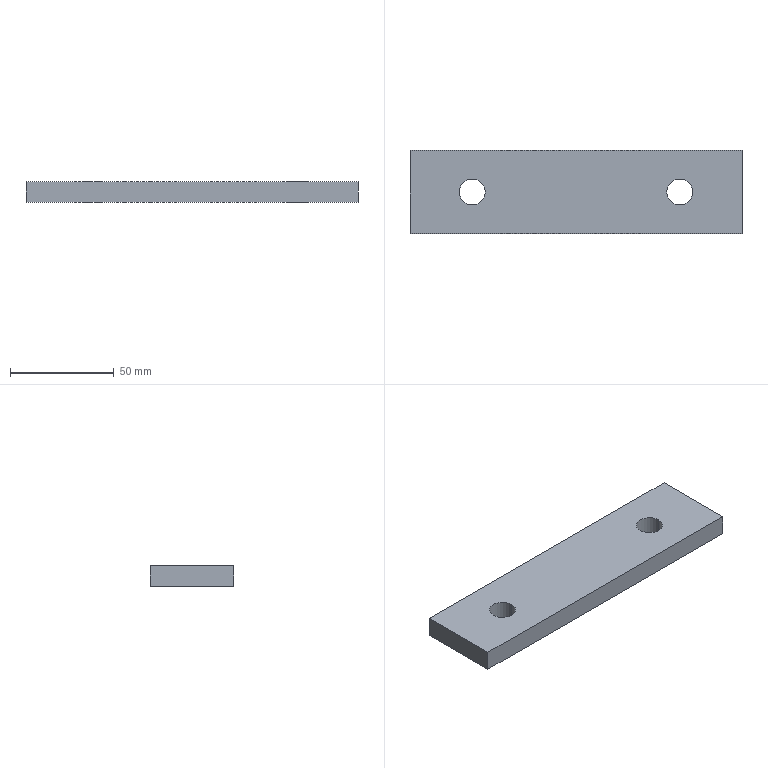Part | SolidWorks | features HoleWzd 2, Extrusion 1 | 1 solid | 10 faces | box 160 x 40 x 10 mm | volume 61546 mm3 | plane 6 | cylinder 4 | commonest cylinder face diameters 12.5 x4
STEP:
#1=CARTESIAN_POINT('',(-56.25,0.,-5.));
#2=VERTEX_POINT('',#1);
#3=CARTESIAN_POINT('',(-43.75,0.,-5.));
#4=VERTEX_POINT('',#3);
#5=CARTESIAN_POINT('',(-50.,0.,-5.));
#6=DIRECTION('',(0.,0.,1.));
#7=DIRECTION('',(1.,0.,0.));
#8=AXIS2_PLACEMENT_3D('',#5,#6,#7);
#9=CIRCLE('',#8,6.25);
#10=EDGE_CURVE('',#2,#4,#9,.T.);
#11=ORIENTED_EDGE('',*,*,#10,.F.);
#12=CARTESIAN_POINT('',(-56.25,0.,5.));
#13=VERTEX_POINT('',#12);
#14=CARTESIAN_POINT('',(-56.25,0.,5.));
#15=DIRECTION('',(0.,0.,1.));
#16=VECTOR('',#15,1000.);
#17=LINE('',#14,#16);
#18=EDGE_CURVE('',#2,#13,#17,.T.);
#19=ORIENTED_EDGE('',*,*,#18,.T.);
#20=CARTESIAN_POINT('',(-43.75,0.,5.));
#21=VERTEX_POINT('',#20);
#22=CARTESIAN_POINT('',(-50.,0.,5.));
#23=DIRECTION('',(0.,0.,1.));
#24=DIRECTION('',(1.,0.,0.));
#25=AXIS2_PLACEMENT_3D('',#22,#23,#24);
#26=CIRCLE('',#25,6.25);
#27=EDGE_CURVE('',#13,#21,#26,.T.);
#28=ORIENTED_EDGE('',*,*,#27,.T.);
#29=CARTESIAN_POINT('',(-43.75,0.,5.));
#30=DIRECTION('',(0.,0.,1.));
#31=VECTOR('',#30,1000.);
#32=LINE('',#29,#31);
#33=EDGE_CURVE('',#4,#21,#32,.T.);
#34=ORIENTED_EDGE('',*,*,#33,.F.);
#35=EDGE_LOOP('',(#11,#19,#28,#34));
#36=FACE_OUTER_BOUND('',#35,.T.);
#37=CARTESIAN_POINT('',(-50.,0.,5.));
#38=DIRECTION('',(0.,0.,1.));
#39=DIRECTION('',(1.,0.,0.));
#40=AXIS2_PLACEMENT_3D('',#37,#38,#39);
#41=CYLINDRICAL_SURFACE('',#40,6.25);
#42=ADVANCED_FACE('',(#36),#41,.F.);
#43=CARTESIAN_POINT('',(43.75,0.,-5.));
#44=VERTEX_POINT('',#43);
#45=CARTESIAN_POINT('',(56.25,0.,-5.));
#46=VERTEX_POINT('',#45);
#47=CARTESIAN_POINT('',(50.,0.,-5.));
#48=DIRECTION('',(0.,0.,1.));
#49=DIRECTION('',(1.,0.,0.));
#50=AXIS2_PLACEMENT_3D('',#47,#48,#49);
#51=CIRCLE('',#50,6.25);
#52=EDGE_CURVE('',#44,#46,#51,.T.);
#53=ORIENTED_EDGE('',*,*,#52,.F.);
#54=CARTESIAN_POINT('',(43.75,0.,5.));
#55=VERTEX_POINT('',#54);
#56=CARTESIAN_POINT('',(43.75,0.,5.));
#57=DIRECTION('',(0.,0.,1.));
#58=VECTOR('',#57,1000.);
#59=LINE('',#56,#58);
#60=EDGE_CURVE('',#44,#55,#59,.T.);
#61=ORIENTED_EDGE('',*,*,#60,.T.);
#62=CARTESIAN_POINT('',(56.25,0.,5.));
#63=VERTEX_POINT('',#62);
#64=CARTESIAN_POINT('',(50.,0.,5.));
#65=DIRECTION('',(0.,0.,1.));
#66=DIRECTION('',(1.,0.,0.));
#67=AXIS2_PLACEMENT_3D('',#64,#65,#66);
#68=CIRCLE('',#67,6.25);
#69=EDGE_CURVE('',#55,#63,#68,.T.);
#70=ORIENTED_EDGE('',*,*,#69,.T.);
#71=CARTESIAN_POINT('',(56.25,0.,5.));
#72=DIRECTION('',(0.,0.,1.));
#73=VECTOR('',#72,1000.);
#74=LINE('',#71,#73);
#75=EDGE_CURVE('',#46,#63,#74,.T.);
#76=ORIENTED_EDGE('',*,*,#75,.F.);
#77=EDGE_LOOP('',(#53,#61,#70,#76));
#78=FACE_OUTER_BOUND('',#77,.T.);
#79=CARTESIAN_POINT('',(50.,0.,5.));
#80=DIRECTION('',(0.,0.,1.));
#81=DIRECTION('',(1.,0.,0.));
#82=AXIS2_PLACEMENT_3D('',#79,#80,#81);
#83=CYLINDRICAL_SURFACE('',#82,6.25);
#84=ADVANCED_FACE('',(#78),#83,.F.);
#85=CARTESIAN_POINT('',(-80.,20.,-5.));
#86=VERTEX_POINT('',#85);
#87=CARTESIAN_POINT('',(-80.,-20.,-5.));
#88=VERTEX_POINT('',#87);
#89=CARTESIAN_POINT('',(-80.,-20.,-5.));
#90=DIRECTION('',(0.,-1.,0.));
#91=VECTOR('',#90,1000.);
#92=LINE('',#89,#91);
#93=EDGE_CURVE('',#86,#88,#92,.T.);
#94=ORIENTED_EDGE('',*,*,#93,.T.);
#95=CARTESIAN_POINT('',(-80.,-20.,5.));
#96=VERTEX_POINT('',#95);
#97=CARTESIAN_POINT('',(-80.,-20.,5.));
#98=DIRECTION('',(0.,0.,-1.));
#99=VECTOR('',#98,1000.);
#100=LINE('',#97,#99);
#101=EDGE_CURVE('',#96,#88,#100,.T.);
#102=ORIENTED_EDGE('',*,*,#101,.F.);
#103=CARTESIAN_POINT('',(-80.,20.,5.));
#104=VERTEX_POINT('',#103);
#105=CARTESIAN_POINT('',(-80.,-20.,5.));
#106=DIRECTION('',(0.,-1.,0.));
#107=VECTOR('',#106,1000.);
#108=LINE('',#105,#107);
#109=EDGE_CURVE('',#104,#96,#108,.T.);
#110=ORIENTED_EDGE('',*,*,#109,.F.);
#111=CARTESIAN_POINT('',(-80.,20.,5.));
#112=DIRECTION('',(0.,0.,-1.));
#113=VECTOR('',#112,1000.);
#114=LINE('',#111,#113);
#115=EDGE_CURVE('',#104,#86,#114,.T.);
#116=ORIENTED_EDGE('',*,*,#115,.T.);
#117=EDGE_LOOP('',(#94,#102,#110,#116));
#118=FACE_OUTER_BOUND('',#117,.T.);
#119=CARTESIAN_POINT('',(-80.,-20.,5.));
#120=DIRECTION('',(1.,0.,0.));
#121=DIRECTION('',(0.,0.,-1.));
#122=AXIS2_PLACEMENT_3D('',#119,#120,#121);
#123=PLANE('',#122);
#124=ADVANCED_FACE('',(#118),#123,.F.);
#125=CARTESIAN_POINT('',(80.,-20.,-5.));
#126=VERTEX_POINT('',#125);
#127=CARTESIAN_POINT('',(80.,-20.,-5.));
#128=DIRECTION('',(1.,0.,0.));
#129=VECTOR('',#128,1000.);
#130=LINE('',#127,#129);
#131=EDGE_CURVE('',#88,#126,#130,.T.);
#132=ORIENTED_EDGE('',*,*,#131,.T.);
#133=CARTESIAN_POINT('',(80.,-20.,5.));
#134=VERTEX_POINT('',#133);
#135=CARTESIAN_POINT('',(80.,-20.,5.));
#136=DIRECTION('',(0.,0.,-1.));
#137=VECTOR('',#136,1000.);
#138=LINE('',#135,#137);
#139=EDGE_CURVE('',#134,#126,#138,.T.);
#140=ORIENTED_EDGE('',*,*,#139,.F.);
#141=CARTESIAN_POINT('',(80.,-20.,5.));
#142=DIRECTION('',(1.,0.,0.));
#143=VECTOR('',#142,1000.);
#144=LINE('',#141,#143);
#145=EDGE_CURVE('',#96,#134,#144,.T.);
#146=ORIENTED_EDGE('',*,*,#145,.F.);
#147=ORIENTED_EDGE('',*,*,#101,.T.);
#148=EDGE_LOOP('',(#132,#140,#146,#147));
#149=FACE_OUTER_BOUND('',#148,.T.);
#150=CARTESIAN_POINT('',(80.,-20.,5.));
#151=DIRECTION('',(0.,1.,0.));
#152=DIRECTION('',(-1.,0.,0.));
#153=AXIS2_PLACEMENT_3D('',#150,#151,#152);
#154=PLANE('',#153);
#155=ADVANCED_FACE('',(#149),#154,.F.);
#156=CARTESIAN_POINT('',(80.,20.,-5.));
#157=VERTEX_POINT('',#156);
#158=CARTESIAN_POINT('',(80.,-20.,-5.));
#159=DIRECTION('',(0.,1.,0.));
#160=VECTOR('',#159,1000.);
#161=LINE('',#158,#160);
#162=EDGE_CURVE('',#126,#157,#161,.T.);
#163=ORIENTED_EDGE('',*,*,#162,.T.);
#164=CARTESIAN_POINT('',(80.,20.,5.));
#165=VERTEX_POINT('',#164);
#166=CARTESIAN_POINT('',(80.,20.,5.));
#167=DIRECTION('',(0.,0.,-1.));
#168=VECTOR('',#167,1000.);
#169=LINE('',#166,#168);
#170=EDGE_CURVE('',#165,#157,#169,.T.);
#171=ORIENTED_EDGE('',*,*,#170,.F.);
#172=CARTESIAN_POINT('',(80.,-20.,5.));
#173=DIRECTION('',(0.,1.,0.));
#174=VECTOR('',#173,1000.);
#175=LINE('',#172,#174);
#176=EDGE_CURVE('',#134,#165,#175,.T.);
#177=ORIENTED_EDGE('',*,*,#176,.F.);
#178=ORIENTED_EDGE('',*,*,#139,.T.);
#179=EDGE_LOOP('',(#163,#171,#177,#178));
#180=FACE_OUTER_BOUND('',#179,.T.);
#181=CARTESIAN_POINT('',(80.,-20.,5.));
#182=DIRECTION('',(-1.,0.,0.));
#183=DIRECTION('',(0.,0.,1.));
#184=AXIS2_PLACEMENT_3D('',#181,#182,#183);
#185=PLANE('',#184);
#186=ADVANCED_FACE('',(#180),#185,.F.);
#187=CARTESIAN_POINT('',(80.,20.,-5.));
#188=DIRECTION('',(-1.,0.,0.));
#189=VECTOR('',#188,1000.);
#190=LINE('',#187,#189);
#191=EDGE_CURVE('',#157,#86,#190,.T.);
#192=ORIENTED_EDGE('',*,*,#191,.T.);
#193=ORIENTED_EDGE('',*,*,#115,.F.);
#194=CARTESIAN_POINT('',(80.,20.,5.));
#195=DIRECTION('',(-1.,0.,0.));
#196=VECTOR('',#195,1000.);
#197=LINE('',#194,#196);
#198=EDGE_CURVE('',#165,#104,#197,.T.);
#199=ORIENTED_EDGE('',*,*,#198,.F.);
#200=ORIENTED_EDGE('',*,*,#170,.T.);
#201=EDGE_LOOP('',(#192,#193,#199,#200));
#202=FACE_OUTER_BOUND('',#201,.T.);
#203=CARTESIAN_POINT('',(80.,20.,5.));
#204=DIRECTION('',(0.,-1.,0.));
#205=DIRECTION('',(1.,0.,0.));
#206=AXIS2_PLACEMENT_3D('',#203,#204,#205);
#207=PLANE('',#206);
#208=ADVANCED_FACE('',(#202),#207,.F.);
#209=CARTESIAN_POINT('',(-50.,0.,5.));
#210=DIRECTION('',(0.,0.,1.));
#211=DIRECTION('',(1.,0.,0.));
#212=AXIS2_PLACEMENT_3D('',#209,#210,#211);
#213=CIRCLE('',#212,6.25);
#214=EDGE_CURVE('',#21,#13,#213,.T.);
#215=ORIENTED_EDGE('',*,*,#214,.F.);
#216=ORIENTED_EDGE('',*,*,#27,.F.);
#217=EDGE_LOOP('',(#215,#216));
#218=FACE_BOUND('',#217,.T.);
#219=CARTESIAN_POINT('',(50.,0.,5.));
#220=DIRECTION('',(0.,0.,1.));
#221=DIRECTION('',(1.,0.,0.));
#222=AXIS2_PLACEMENT_3D('',#219,#220,#221);
#223=CIRCLE('',#222,6.25);
#224=EDGE_CURVE('',#63,#55,#223,.T.);
#225=ORIENTED_EDGE('',*,*,#224,.F.);
#226=ORIENTED_EDGE('',*,*,#69,.F.);
#227=EDGE_LOOP('',(#225,#226));
#228=FACE_BOUND('',#227,.T.);
#229=ORIENTED_EDGE('',*,*,#109,.T.);
#230=ORIENTED_EDGE('',*,*,#145,.T.);
#231=ORIENTED_EDGE('',*,*,#176,.T.);
#232=ORIENTED_EDGE('',*,*,#198,.T.);
#233=EDGE_LOOP('',(#229,#230,#231,#232));
#234=FACE_OUTER_BOUND('',#233,.T.);
#235=CARTESIAN_POINT('',(0.,0.,5.));
#236=DIRECTION('',(0.,0.,1.));
#237=DIRECTION('',(1.,0.,0.));
#238=AXIS2_PLACEMENT_3D('',#235,#236,#237);
#239=PLANE('',#238);
#240=ADVANCED_FACE('',(#218,#228,#234),#239,.T.);
#241=CARTESIAN_POINT('',(-50.,0.,-5.));
#242=DIRECTION('',(0.,0.,1.));
#243=DIRECTION('',(1.,0.,0.));
#244=AXIS2_PLACEMENT_3D('',#241,#242,#243);
#245=CIRCLE('',#244,6.25);
#246=EDGE_CURVE('',#4,#2,#245,.T.);
#247=ORIENTED_EDGE('',*,*,#246,.T.);
#248=ORIENTED_EDGE('',*,*,#10,.T.);
#249=EDGE_LOOP('',(#247,#248));
#250=FACE_BOUND('',#249,.T.);
#251=CARTESIAN_POINT('',(50.,0.,-5.));
#252=DIRECTION('',(0.,0.,1.));
#253=DIRECTION('',(1.,0.,0.));
#254=AXIS2_PLACEMENT_3D('',#251,#252,#253);
#255=CIRCLE('',#254,6.25);
#256=EDGE_CURVE('',#46,#44,#255,.T.);
#257=ORIENTED_EDGE('',*,*,#256,.T.);
#258=ORIENTED_EDGE('',*,*,#52,.T.);
#259=EDGE_LOOP('',(#257,#258));
#260=FACE_BOUND('',#259,.T.);
#261=ORIENTED_EDGE('',*,*,#93,.F.);
#262=ORIENTED_EDGE('',*,*,#191,.F.);
#263=ORIENTED_EDGE('',*,*,#162,.F.);
#264=ORIENTED_EDGE('',*,*,#131,.F.);
#265=EDGE_LOOP('',(#261,#262,#263,#264));
#266=FACE_OUTER_BOUND('',#265,.T.);
#267=CARTESIAN_POINT('',(0.,0.,-5.));
#268=DIRECTION('',(0.,0.,1.));
#269=DIRECTION('',(1.,0.,0.));
#270=AXIS2_PLACEMENT_3D('',#267,#268,#269);
#271=PLANE('',#270);
#272=ADVANCED_FACE('',(#250,#260,#266),#271,.F.);
#273=ORIENTED_EDGE('',*,*,#60,.F.);
#274=ORIENTED_EDGE('',*,*,#256,.F.);
#275=ORIENTED_EDGE('',*,*,#75,.T.);
#276=ORIENTED_EDGE('',*,*,#224,.T.);
#277=EDGE_LOOP('',(#273,#274,#275,#276));
#278=FACE_OUTER_BOUND('',#277,.T.);
#279=CARTESIAN_POINT('',(50.,0.,5.));
#280=DIRECTION('',(0.,0.,1.));
#281=DIRECTION('',(1.,0.,0.));
#282=AXIS2_PLACEMENT_3D('',#279,#280,#281);
#283=CYLINDRICAL_SURFACE('',#282,6.25);
#284=ADVANCED_FACE('',(#278),#283,.F.);
#285=ORIENTED_EDGE('',*,*,#18,.F.);
#286=ORIENTED_EDGE('',*,*,#246,.F.);
#287=ORIENTED_EDGE('',*,*,#33,.T.);
#288=ORIENTED_EDGE('',*,*,#214,.T.);
#289=EDGE_LOOP('',(#285,#286,#287,#288));
#290=FACE_OUTER_BOUND('',#289,.T.);
#291=CARTESIAN_POINT('',(-50.,0.,5.));
#292=DIRECTION('',(0.,0.,1.));
#293=DIRECTION('',(1.,0.,0.));
#294=AXIS2_PLACEMENT_3D('',#291,#292,#293);
#295=CYLINDRICAL_SURFACE('',#294,6.25);
#296=ADVANCED_FACE('',(#290),#295,.F.);
#297=CLOSED_SHELL('',(#42,#84,#124,#155,#186,#208,#240,#272,#284,#296));
#298=MANIFOLD_SOLID_BREP('',#297);
#299=CARTESIAN_POINT('',(0.,0.,0.));
#300=DIRECTION('',(0.,0.,1.));
#301=DIRECTION('',(1.,0.,0.));
#302=AXIS2_PLACEMENT_3D('',#299,#300,#301);
#303=(LENGTH_UNIT()NAMED_UNIT(*)SI_UNIT(.MILLI.,.METRE.));
#304=UNCERTAINTY_MEASURE_WITH_UNIT(LENGTH_MEASURE(0.00001),#303,'','');
#305=(NAMED_UNIT(*)PLANE_ANGLE_UNIT()SI_UNIT($,.RADIAN.));
#306=(NAMED_UNIT(*)SI_UNIT($,.STERADIAN.)SOLID_ANGLE_UNIT());
#307=(GEOMETRIC_REPRESENTATION_CONTEXT(3)GLOBAL_UNCERTAINTY_ASSIGNED_CONTEXT((#304))GLOBAL_UNIT_ASSIGNED_CONTEXT((#303,#305,#306))REPRESENTATION_CONTEXT('',''));
#308=ADVANCED_BREP_SHAPE_REPRESENTATION('',(#298,#302),#307);